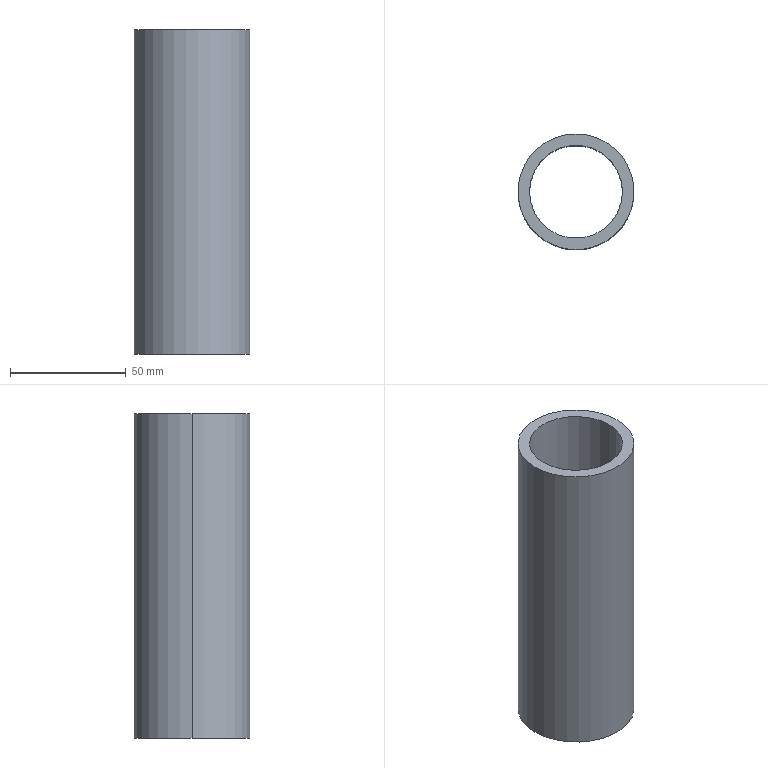Part | STEP file | LM-05-1229_default | 1 solid | 6 faces | box 50 x 50 x 140 mm | volume 98079 mm3 | cylinder 4 | plane 2 | commonest cylinder face diameters 40.1 x2 50 x2
STEP:
#1=CARTESIAN_POINT('',(0.,0.,0.));
#2=DIRECTION('',(0.,0.,1.));
#3=DIRECTION('',(1.,0.,0.));
#4=AXIS2_PLACEMENT_3D('',#1,#2,#3);
#5=CARTESIAN_POINT('',(-20.05,0.,70.));
#6=VERTEX_POINT('',#5);
#7=CARTESIAN_POINT('',(-20.05,0.,-70.));
#8=VERTEX_POINT('',#7);
#9=CARTESIAN_POINT('',(-20.05,0.,70.));
#10=DIRECTION('',(0.,0.,-1.));
#11=VECTOR('',#10,1.);
#12=LINE('',#9,#11);
#13=CARTESIAN_POINT('',(0.,0.,70.));
#14=DIRECTION('',(0.,0.,-1.));
#15=DIRECTION('',(-1.,0.,0.));
#16=AXIS2_PLACEMENT_3D('',#13,#14,#15);
#17=CYLINDRICAL_SURFACE('',#16,20.05);
#18=CARTESIAN_POINT('',(6.283,0.));
#19=DIRECTION('',(0.,1.));
#20=VECTOR('',#19,1.);
#21=LINE('',#18,#20);
#22=(GEOMETRIC_REPRESENTATION_CONTEXT(2)PARAMETRIC_REPRESENTATION_CONTEXT()REPRESENTATION_CONTEXT('',''));
#23=DEFINITIONAL_REPRESENTATION('',(#21),#22);
#24=PCURVE('',#17,#23);
#25=CARTESIAN_POINT('',(0.,0.,70.));
#26=DIRECTION('',(0.,0.,-1.));
#27=DIRECTION('',(-1.,0.,0.));
#28=AXIS2_PLACEMENT_3D('',#25,#26,#27);
#29=CYLINDRICAL_SURFACE('',#28,20.05);
#30=CARTESIAN_POINT('',(0.,0.));
#31=DIRECTION('',(0.,1.));
#32=VECTOR('',#31,1.);
#33=LINE('',#30,#32);
#34=(GEOMETRIC_REPRESENTATION_CONTEXT(2)PARAMETRIC_REPRESENTATION_CONTEXT()REPRESENTATION_CONTEXT('',''));
#35=DEFINITIONAL_REPRESENTATION('',(#33),#34);
#36=PCURVE('',#29,#35);
#37=SURFACE_CURVE('',#12,(#24,#36),.PCURVE_S1.);
#38=EDGE_CURVE('',#6,#8,#37,.T.);
#39=ORIENTED_EDGE('',*,*,#38,.T.);
#40=CARTESIAN_POINT('',(20.05,0.,-70.));
#41=VERTEX_POINT('',#40);
#42=CARTESIAN_POINT('',(0.,0.,-70.));
#43=DIRECTION('',(0.,0.,1.));
#44=DIRECTION('',(1.,0.,0.));
#45=AXIS2_PLACEMENT_3D('',#42,#43,#44);
#46=CIRCLE('',#45,20.05);
#47=CARTESIAN_POINT('',(9.425,140.));
#48=DIRECTION('',(-1.,0.));
#49=VECTOR('',#48,1.);
#50=LINE('',#47,#49);
#51=(GEOMETRIC_REPRESENTATION_CONTEXT(2)PARAMETRIC_REPRESENTATION_CONTEXT()REPRESENTATION_CONTEXT('',''));
#52=DEFINITIONAL_REPRESENTATION('',(#50),#51);
#53=PCURVE('',#17,#52);
#54=CARTESIAN_POINT('',(0.,0.,-70.));
#55=DIRECTION('',(0.,0.,1.));
#56=DIRECTION('',(1.,0.,0.));
#57=AXIS2_PLACEMENT_3D('',#54,#55,#56);
#58=PLANE('',#57);
#59=CARTESIAN_POINT('',(0.,0.));
#60=DIRECTION('',(1.,0.));
#61=AXIS2_PLACEMENT_2D('',#59,#60);
#62=CIRCLE('',#61,20.05);
#63=(GEOMETRIC_REPRESENTATION_CONTEXT(2)PARAMETRIC_REPRESENTATION_CONTEXT()REPRESENTATION_CONTEXT('',''));
#64=DEFINITIONAL_REPRESENTATION('',(#62),#63);
#65=PCURVE('',#58,#64);
#66=SURFACE_CURVE('',#46,(#53,#65),.PCURVE_S1.);
#67=EDGE_CURVE('',#8,#41,#66,.T.);
#68=ORIENTED_EDGE('',*,*,#67,.T.);
#69=CARTESIAN_POINT('',(20.05,0.,70.));
#70=VERTEX_POINT('',#69);
#71=CARTESIAN_POINT('',(20.05,0.,70.));
#72=DIRECTION('',(0.,0.,-1.));
#73=VECTOR('',#72,1.);
#74=LINE('',#71,#73);
#75=CARTESIAN_POINT('',(3.142,0.));
#76=DIRECTION('',(0.,1.));
#77=VECTOR('',#76,1.);
#78=LINE('',#75,#77);
#79=(GEOMETRIC_REPRESENTATION_CONTEXT(2)PARAMETRIC_REPRESENTATION_CONTEXT()REPRESENTATION_CONTEXT('',''));
#80=DEFINITIONAL_REPRESENTATION('',(#78),#79);
#81=PCURVE('',#17,#80);
#82=CARTESIAN_POINT('',(3.142,0.));
#83=DIRECTION('',(0.,1.));
#84=VECTOR('',#83,1.);
#85=LINE('',#82,#84);
#86=(GEOMETRIC_REPRESENTATION_CONTEXT(2)PARAMETRIC_REPRESENTATION_CONTEXT()REPRESENTATION_CONTEXT('',''));
#87=DEFINITIONAL_REPRESENTATION('',(#85),#86);
#88=PCURVE('',#29,#87);
#89=SURFACE_CURVE('',#74,(#81,#88),.PCURVE_S1.);
#90=EDGE_CURVE('',#70,#41,#89,.T.);
#91=ORIENTED_EDGE('',*,*,#90,.F.);
#92=CARTESIAN_POINT('',(0.,0.,70.));
#93=DIRECTION('',(0.,0.,1.));
#94=DIRECTION('',(1.,0.,0.));
#95=AXIS2_PLACEMENT_3D('',#92,#93,#94);
#96=CIRCLE('',#95,20.05);
#97=CARTESIAN_POINT('',(9.425,0.));
#98=DIRECTION('',(-1.,0.));
#99=VECTOR('',#98,1.);
#100=LINE('',#97,#99);
#101=(GEOMETRIC_REPRESENTATION_CONTEXT(2)PARAMETRIC_REPRESENTATION_CONTEXT()REPRESENTATION_CONTEXT('',''));
#102=DEFINITIONAL_REPRESENTATION('',(#100),#101);
#103=PCURVE('',#17,#102);
#104=CARTESIAN_POINT('',(0.,0.,70.));
#105=DIRECTION('',(0.,0.,1.));
#106=DIRECTION('',(1.,0.,0.));
#107=AXIS2_PLACEMENT_3D('',#104,#105,#106);
#108=PLANE('',#107);
#109=CARTESIAN_POINT('',(0.,0.));
#110=DIRECTION('',(1.,0.));
#111=AXIS2_PLACEMENT_2D('',#109,#110);
#112=CIRCLE('',#111,20.05);
#113=(GEOMETRIC_REPRESENTATION_CONTEXT(2)PARAMETRIC_REPRESENTATION_CONTEXT()REPRESENTATION_CONTEXT('',''));
#114=DEFINITIONAL_REPRESENTATION('',(#112),#113);
#115=PCURVE('',#108,#114);
#116=SURFACE_CURVE('',#96,(#103,#115),.PCURVE_S1.);
#117=EDGE_CURVE('',#6,#70,#116,.T.);
#118=ORIENTED_EDGE('',*,*,#117,.F.);
#119=EDGE_LOOP('',(#39,#68,#91,#118));
#120=FACE_BOUND('',#119,.F.);
#121=ADVANCED_FACE('',(#120),#17,.F.);
#122=CARTESIAN_POINT('',(25.,0.,70.));
#123=VERTEX_POINT('',#122);
#124=CARTESIAN_POINT('',(-25.,0.,70.));
#125=VERTEX_POINT('',#124);
#126=CARTESIAN_POINT('',(0.,0.,70.));
#127=DIRECTION('',(0.,0.,1.));
#128=DIRECTION('',(1.,0.,0.));
#129=AXIS2_PLACEMENT_3D('',#126,#127,#128);
#130=CIRCLE('',#129,25.);
#131=CARTESIAN_POINT('',(0.,0.,70.));
#132=DIRECTION('',(0.,0.,-1.));
#133=DIRECTION('',(-1.,0.,0.));
#134=AXIS2_PLACEMENT_3D('',#131,#132,#133);
#135=CYLINDRICAL_SURFACE('',#134,25.);
#136=CARTESIAN_POINT('',(3.142,0.));
#137=DIRECTION('',(-1.,0.));
#138=VECTOR('',#137,1.);
#139=LINE('',#136,#138);
#140=(GEOMETRIC_REPRESENTATION_CONTEXT(2)PARAMETRIC_REPRESENTATION_CONTEXT()REPRESENTATION_CONTEXT('',''));
#141=DEFINITIONAL_REPRESENTATION('',(#139),#140);
#142=PCURVE('',#135,#141);
#143=CARTESIAN_POINT('',(0.,0.));
#144=DIRECTION('',(1.,0.));
#145=AXIS2_PLACEMENT_2D('',#143,#144);
#146=CIRCLE('',#145,25.);
#147=(GEOMETRIC_REPRESENTATION_CONTEXT(2)PARAMETRIC_REPRESENTATION_CONTEXT()REPRESENTATION_CONTEXT('',''));
#148=DEFINITIONAL_REPRESENTATION('',(#146),#147);
#149=PCURVE('',#108,#148);
#150=SURFACE_CURVE('',#130,(#142,#149),.PCURVE_S1.);
#151=EDGE_CURVE('',#123,#125,#150,.T.);
#152=ORIENTED_EDGE('',*,*,#151,.F.);
#153=CARTESIAN_POINT('',(25.,0.,-70.));
#154=VERTEX_POINT('',#153);
#155=CARTESIAN_POINT('',(25.,0.,70.));
#156=DIRECTION('',(0.,0.,-1.));
#157=VECTOR('',#156,1.);
#158=LINE('',#155,#157);
#159=CARTESIAN_POINT('',(3.142,0.));
#160=DIRECTION('',(0.,1.));
#161=VECTOR('',#160,1.);
#162=LINE('',#159,#161);
#163=(GEOMETRIC_REPRESENTATION_CONTEXT(2)PARAMETRIC_REPRESENTATION_CONTEXT()REPRESENTATION_CONTEXT('',''));
#164=DEFINITIONAL_REPRESENTATION('',(#162),#163);
#165=PCURVE('',#135,#164);
#166=CARTESIAN_POINT('',(0.,0.,70.));
#167=DIRECTION('',(0.,0.,-1.));
#168=DIRECTION('',(-1.,0.,0.));
#169=AXIS2_PLACEMENT_3D('',#166,#167,#168);
#170=CYLINDRICAL_SURFACE('',#169,25.);
#171=CARTESIAN_POINT('',(3.142,0.));
#172=DIRECTION('',(0.,1.));
#173=VECTOR('',#172,1.);
#174=LINE('',#171,#173);
#175=(GEOMETRIC_REPRESENTATION_CONTEXT(2)PARAMETRIC_REPRESENTATION_CONTEXT()REPRESENTATION_CONTEXT('',''));
#176=DEFINITIONAL_REPRESENTATION('',(#174),#175);
#177=PCURVE('',#170,#176);
#178=SURFACE_CURVE('',#158,(#165,#177),.PCURVE_S1.);
#179=EDGE_CURVE('',#123,#154,#178,.T.);
#180=ORIENTED_EDGE('',*,*,#179,.T.);
#181=CARTESIAN_POINT('',(-25.,0.,-70.));
#182=VERTEX_POINT('',#181);
#183=CARTESIAN_POINT('',(0.,0.,-70.));
#184=DIRECTION('',(0.,0.,1.));
#185=DIRECTION('',(1.,0.,0.));
#186=AXIS2_PLACEMENT_3D('',#183,#184,#185);
#187=CIRCLE('',#186,25.);
#188=CARTESIAN_POINT('',(3.142,140.));
#189=DIRECTION('',(-1.,0.));
#190=VECTOR('',#189,1.);
#191=LINE('',#188,#190);
#192=(GEOMETRIC_REPRESENTATION_CONTEXT(2)PARAMETRIC_REPRESENTATION_CONTEXT()REPRESENTATION_CONTEXT('',''));
#193=DEFINITIONAL_REPRESENTATION('',(#191),#192);
#194=PCURVE('',#135,#193);
#195=CARTESIAN_POINT('',(0.,0.));
#196=DIRECTION('',(1.,0.));
#197=AXIS2_PLACEMENT_2D('',#195,#196);
#198=CIRCLE('',#197,25.);
#199=(GEOMETRIC_REPRESENTATION_CONTEXT(2)PARAMETRIC_REPRESENTATION_CONTEXT()REPRESENTATION_CONTEXT('',''));
#200=DEFINITIONAL_REPRESENTATION('',(#198),#199);
#201=PCURVE('',#58,#200);
#202=SURFACE_CURVE('',#187,(#194,#201),.PCURVE_S1.);
#203=EDGE_CURVE('',#154,#182,#202,.T.);
#204=ORIENTED_EDGE('',*,*,#203,.T.);
#205=CARTESIAN_POINT('',(-25.,0.,70.));
#206=DIRECTION('',(0.,0.,-1.));
#207=VECTOR('',#206,1.);
#208=LINE('',#205,#207);
#209=CARTESIAN_POINT('',(0.,0.));
#210=DIRECTION('',(0.,1.));
#211=VECTOR('',#210,1.);
#212=LINE('',#209,#211);
#213=(GEOMETRIC_REPRESENTATION_CONTEXT(2)PARAMETRIC_REPRESENTATION_CONTEXT()REPRESENTATION_CONTEXT('',''));
#214=DEFINITIONAL_REPRESENTATION('',(#212),#213);
#215=PCURVE('',#135,#214);
#216=CARTESIAN_POINT('',(6.283,0.));
#217=DIRECTION('',(0.,1.));
#218=VECTOR('',#217,1.);
#219=LINE('',#216,#218);
#220=(GEOMETRIC_REPRESENTATION_CONTEXT(2)PARAMETRIC_REPRESENTATION_CONTEXT()REPRESENTATION_CONTEXT('',''));
#221=DEFINITIONAL_REPRESENTATION('',(#219),#220);
#222=PCURVE('',#170,#221);
#223=SURFACE_CURVE('',#208,(#215,#222),.PCURVE_S1.);
#224=EDGE_CURVE('',#125,#182,#223,.T.);
#225=ORIENTED_EDGE('',*,*,#224,.F.);
#226=EDGE_LOOP('',(#152,#180,#204,#225));
#227=FACE_BOUND('',#226,.T.);
#228=ADVANCED_FACE('',(#227),#135,.T.);
#229=CARTESIAN_POINT('',(0.,0.,70.));
#230=DIRECTION('',(0.,0.,1.));
#231=DIRECTION('',(1.,0.,0.));
#232=AXIS2_PLACEMENT_3D('',#229,#230,#231);
#233=CIRCLE('',#232,25.);
#234=CARTESIAN_POINT('',(0.,0.));
#235=DIRECTION('',(1.,0.));
#236=AXIS2_PLACEMENT_2D('',#234,#235);
#237=CIRCLE('',#236,25.);
#238=(GEOMETRIC_REPRESENTATION_CONTEXT(2)PARAMETRIC_REPRESENTATION_CONTEXT()REPRESENTATION_CONTEXT('',''));
#239=DEFINITIONAL_REPRESENTATION('',(#237),#238);
#240=PCURVE('',#108,#239);
#241=CARTESIAN_POINT('',(9.425,0.));
#242=DIRECTION('',(-1.,0.));
#243=VECTOR('',#242,1.);
#244=LINE('',#241,#243);
#245=(GEOMETRIC_REPRESENTATION_CONTEXT(2)PARAMETRIC_REPRESENTATION_CONTEXT()REPRESENTATION_CONTEXT('',''));
#246=DEFINITIONAL_REPRESENTATION('',(#244),#245);
#247=PCURVE('',#170,#246);
#248=SURFACE_CURVE('',#233,(#240,#247),.PCURVE_S1.);
#249=EDGE_CURVE('',#125,#123,#248,.T.);
#250=ORIENTED_EDGE('',*,*,#249,.T.);
#251=ORIENTED_EDGE('',*,*,#151,.T.);
#252=EDGE_LOOP('',(#250,#251));
#253=FACE_BOUND('',#252,.T.);
#254=ORIENTED_EDGE('',*,*,#117,.F.);
#255=CARTESIAN_POINT('',(0.,0.,70.));
#256=DIRECTION('',(0.,0.,1.));
#257=DIRECTION('',(1.,0.,0.));
#258=AXIS2_PLACEMENT_3D('',#255,#256,#257);
#259=CIRCLE('',#258,20.05);
#260=CARTESIAN_POINT('',(0.,0.));
#261=DIRECTION('',(1.,0.));
#262=AXIS2_PLACEMENT_2D('',#260,#261);
#263=CIRCLE('',#262,20.05);
#264=(GEOMETRIC_REPRESENTATION_CONTEXT(2)PARAMETRIC_REPRESENTATION_CONTEXT()REPRESENTATION_CONTEXT('',''));
#265=DEFINITIONAL_REPRESENTATION('',(#263),#264);
#266=PCURVE('',#108,#265);
#267=CARTESIAN_POINT('',(3.142,0.));
#268=DIRECTION('',(-1.,0.));
#269=VECTOR('',#268,1.);
#270=LINE('',#267,#269);
#271=(GEOMETRIC_REPRESENTATION_CONTEXT(2)PARAMETRIC_REPRESENTATION_CONTEXT()REPRESENTATION_CONTEXT('',''));
#272=DEFINITIONAL_REPRESENTATION('',(#270),#271);
#273=PCURVE('',#29,#272);
#274=SURFACE_CURVE('',#259,(#266,#273),.PCURVE_S1.);
#275=EDGE_CURVE('',#70,#6,#274,.T.);
#276=ORIENTED_EDGE('',*,*,#275,.F.);
#277=EDGE_LOOP('',(#254,#276));
#278=FACE_BOUND('',#277,.T.);
#279=ADVANCED_FACE('',(#253,#278),#108,.T.);
#280=CARTESIAN_POINT('',(0.,0.,-70.));
#281=DIRECTION('',(0.,0.,1.));
#282=DIRECTION('',(1.,0.,0.));
#283=AXIS2_PLACEMENT_3D('',#280,#281,#282);
#284=CIRCLE('',#283,25.);
#285=CARTESIAN_POINT('',(0.,0.));
#286=DIRECTION('',(1.,0.));
#287=AXIS2_PLACEMENT_2D('',#285,#286);
#288=CIRCLE('',#287,25.);
#289=(GEOMETRIC_REPRESENTATION_CONTEXT(2)PARAMETRIC_REPRESENTATION_CONTEXT()REPRESENTATION_CONTEXT('',''));
#290=DEFINITIONAL_REPRESENTATION('',(#288),#289);
#291=PCURVE('',#58,#290);
#292=CARTESIAN_POINT('',(9.425,140.));
#293=DIRECTION('',(-1.,0.));
#294=VECTOR('',#293,1.);
#295=LINE('',#292,#294);
#296=(GEOMETRIC_REPRESENTATION_CONTEXT(2)PARAMETRIC_REPRESENTATION_CONTEXT()REPRESENTATION_CONTEXT('',''));
#297=DEFINITIONAL_REPRESENTATION('',(#295),#296);
#298=PCURVE('',#170,#297);
#299=SURFACE_CURVE('',#284,(#291,#298),.PCURVE_S1.);
#300=EDGE_CURVE('',#182,#154,#299,.T.);
#301=ORIENTED_EDGE('',*,*,#300,.F.);
#302=ORIENTED_EDGE('',*,*,#203,.F.);
#303=EDGE_LOOP('',(#301,#302));
#304=FACE_BOUND('',#303,.T.);
#305=ORIENTED_EDGE('',*,*,#67,.T.);
#306=CARTESIAN_POINT('',(0.,0.,-70.));
#307=DIRECTION('',(0.,0.,1.));
#308=DIRECTION('',(1.,0.,0.));
#309=AXIS2_PLACEMENT_3D('',#306,#307,#308);
#310=CIRCLE('',#309,20.05);
#311=CARTESIAN_POINT('',(0.,0.));
#312=DIRECTION('',(1.,0.));
#313=AXIS2_PLACEMENT_2D('',#311,#312);
#314=CIRCLE('',#313,20.05);
#315=(GEOMETRIC_REPRESENTATION_CONTEXT(2)PARAMETRIC_REPRESENTATION_CONTEXT()REPRESENTATION_CONTEXT('',''));
#316=DEFINITIONAL_REPRESENTATION('',(#314),#315);
#317=PCURVE('',#58,#316);
#318=CARTESIAN_POINT('',(3.142,140.));
#319=DIRECTION('',(-1.,0.));
#320=VECTOR('',#319,1.);
#321=LINE('',#318,#320);
#322=(GEOMETRIC_REPRESENTATION_CONTEXT(2)PARAMETRIC_REPRESENTATION_CONTEXT()REPRESENTATION_CONTEXT('',''));
#323=DEFINITIONAL_REPRESENTATION('',(#321),#322);
#324=PCURVE('',#29,#323);
#325=SURFACE_CURVE('',#310,(#317,#324),.PCURVE_S1.);
#326=EDGE_CURVE('',#41,#8,#325,.T.);
#327=ORIENTED_EDGE('',*,*,#326,.T.);
#328=EDGE_LOOP('',(#305,#327));
#329=FACE_BOUND('',#328,.T.);
#330=ADVANCED_FACE('',(#304,#329),#58,.F.);
#331=ORIENTED_EDGE('',*,*,#179,.F.);
#332=ORIENTED_EDGE('',*,*,#249,.F.);
#333=ORIENTED_EDGE('',*,*,#224,.T.);
#334=ORIENTED_EDGE('',*,*,#300,.T.);
#335=EDGE_LOOP('',(#331,#332,#333,#334));
#336=FACE_BOUND('',#335,.T.);
#337=ADVANCED_FACE('',(#336),#170,.T.);
#338=ORIENTED_EDGE('',*,*,#326,.T.);
#339=ORIENTED_EDGE('',*,*,#38,.F.);
#340=ORIENTED_EDGE('',*,*,#275,.F.);
#341=ORIENTED_EDGE('',*,*,#90,.T.);
#342=EDGE_LOOP('',(#338,#339,#340,#341));
#343=FACE_BOUND('',#342,.F.);
#344=ADVANCED_FACE('',(#343),#29,.F.);
#345=CLOSED_SHELL('',(#121,#228,#279,#330,#337,#344));
#346=MANIFOLD_SOLID_BREP('',#345);
#347=(LENGTH_UNIT()NAMED_UNIT(*)SI_UNIT(.MILLI.,.METRE.));
#348=UNCERTAINTY_MEASURE_WITH_UNIT(LENGTH_MEASURE(0.0000001),#347,'','');
#349=(NAMED_UNIT(*)PLANE_ANGLE_UNIT()SI_UNIT($,.RADIAN.));
#350=(NAMED_UNIT(*)SI_UNIT($,.STERADIAN.)SOLID_ANGLE_UNIT());
#351=(GEOMETRIC_REPRESENTATION_CONTEXT(3)GLOBAL_UNCERTAINTY_ASSIGNED_CONTEXT((#348))GLOBAL_UNIT_ASSIGNED_CONTEXT((#347,#349,#350))REPRESENTATION_CONTEXT('',''));
#352=ADVANCED_BREP_SHAPE_REPRESENTATION('',(#4,#346),#351);